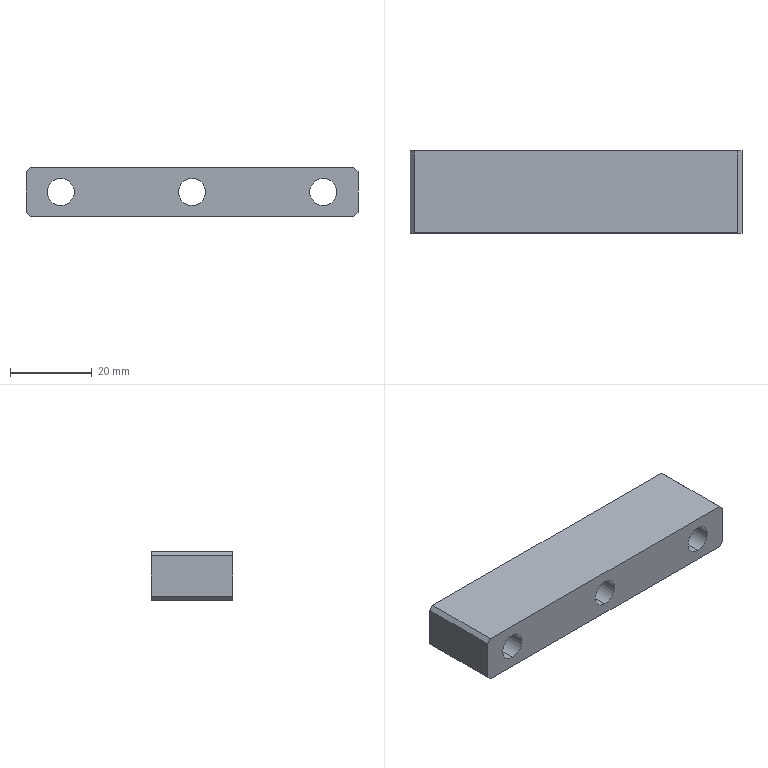Part | SolidWorks | features Chamfer 1, Extrusion 1, HoleWzd 1 | 1 solid | 25 faces | box 81 x 20 x 12 mm | volume 16180 mm3 | plane 13 | cylinder 12 | commonest cylinder face diameters 6.6 x6 11 x6
STEP:
#1=CARTESIAN_POINT('',(-32.,3.6,0.5));
#2=VERTEX_POINT('',#1);
#3=CARTESIAN_POINT('',(-32.,3.6,11.5));
#4=VERTEX_POINT('',#3);
#5=CARTESIAN_POINT('',(-32.,3.6,6.));
#6=DIRECTION('',(0.,1.,0.));
#7=DIRECTION('',(0.,0.,1.));
#8=AXIS2_PLACEMENT_3D('',#5,#6,#7);
#9=CIRCLE('',#8,5.5);
#10=EDGE_CURVE('',#2,#4,#9,.T.);
#11=ORIENTED_EDGE('',*,*,#10,.F.);
#12=CARTESIAN_POINT('',(-32.,10.,0.5));
#13=VERTEX_POINT('',#12);
#14=CARTESIAN_POINT('',(-32.,10.,0.5));
#15=DIRECTION('',(0.,1.,0.));
#16=VECTOR('',#15,1000.);
#17=LINE('',#14,#16);
#18=EDGE_CURVE('',#2,#13,#17,.T.);
#19=ORIENTED_EDGE('',*,*,#18,.T.);
#20=CARTESIAN_POINT('',(-32.,10.,11.5));
#21=VERTEX_POINT('',#20);
#22=CARTESIAN_POINT('',(-32.,10.,6.));
#23=DIRECTION('',(0.,1.,0.));
#24=DIRECTION('',(0.,0.,1.));
#25=AXIS2_PLACEMENT_3D('',#22,#23,#24);
#26=CIRCLE('',#25,5.5);
#27=EDGE_CURVE('',#13,#21,#26,.T.);
#28=ORIENTED_EDGE('',*,*,#27,.T.);
#29=CARTESIAN_POINT('',(-32.,10.,11.5));
#30=DIRECTION('',(0.,1.,0.));
#31=VECTOR('',#30,1000.);
#32=LINE('',#29,#31);
#33=EDGE_CURVE('',#4,#21,#32,.T.);
#34=ORIENTED_EDGE('',*,*,#33,.F.);
#35=EDGE_LOOP('',(#11,#19,#28,#34));
#36=FACE_OUTER_BOUND('',#35,.T.);
#37=CARTESIAN_POINT('',(-32.,10.,6.));
#38=DIRECTION('',(0.,1.,0.));
#39=DIRECTION('',(0.,0.,1.));
#40=AXIS2_PLACEMENT_3D('',#37,#38,#39);
#41=CYLINDRICAL_SURFACE('',#40,5.5);
#42=ADVANCED_FACE('',(#36),#41,.F.);
#43=CARTESIAN_POINT('',(-32.,-10.,2.7));
#44=VERTEX_POINT('',#43);
#45=CARTESIAN_POINT('',(-32.,-10.,9.3));
#46=VERTEX_POINT('',#45);
#47=CARTESIAN_POINT('',(-32.,-10.,6.));
#48=DIRECTION('',(0.,1.,0.));
#49=DIRECTION('',(0.,0.,1.));
#50=AXIS2_PLACEMENT_3D('',#47,#48,#49);
#51=CIRCLE('',#50,3.3);
#52=EDGE_CURVE('',#44,#46,#51,.T.);
#53=ORIENTED_EDGE('',*,*,#52,.F.);
#54=CARTESIAN_POINT('',(-32.,3.6,2.7));
#55=VERTEX_POINT('',#54);
#56=CARTESIAN_POINT('',(-32.,10.,2.7));
#57=DIRECTION('',(0.,1.,0.));
#58=VECTOR('',#57,1000.);
#59=LINE('',#56,#58);
#60=EDGE_CURVE('',#44,#55,#59,.T.);
#61=ORIENTED_EDGE('',*,*,#60,.T.);
#62=CARTESIAN_POINT('',(-32.,3.6,9.3));
#63=VERTEX_POINT('',#62);
#64=CARTESIAN_POINT('',(-32.,3.6,6.));
#65=DIRECTION('',(0.,1.,0.));
#66=DIRECTION('',(0.,0.,1.));
#67=AXIS2_PLACEMENT_3D('',#64,#65,#66);
#68=CIRCLE('',#67,3.3);
#69=EDGE_CURVE('',#55,#63,#68,.T.);
#70=ORIENTED_EDGE('',*,*,#69,.T.);
#71=CARTESIAN_POINT('',(-32.,10.,9.3));
#72=DIRECTION('',(0.,1.,0.));
#73=VECTOR('',#72,1000.);
#74=LINE('',#71,#73);
#75=EDGE_CURVE('',#46,#63,#74,.T.);
#76=ORIENTED_EDGE('',*,*,#75,.F.);
#77=EDGE_LOOP('',(#53,#61,#70,#76));
#78=FACE_OUTER_BOUND('',#77,.T.);
#79=CARTESIAN_POINT('',(-32.,10.,6.));
#80=DIRECTION('',(0.,1.,0.));
#81=DIRECTION('',(0.,0.,1.));
#82=AXIS2_PLACEMENT_3D('',#79,#80,#81);
#83=CYLINDRICAL_SURFACE('',#82,3.3);
#84=ADVANCED_FACE('',(#78),#83,.F.);
#85=CARTESIAN_POINT('',(0.,3.6,0.5));
#86=VERTEX_POINT('',#85);
#87=CARTESIAN_POINT('',(0.,3.6,11.5));
#88=VERTEX_POINT('',#87);
#89=CARTESIAN_POINT('',(0.,3.6,6.));
#90=DIRECTION('',(0.,1.,0.));
#91=DIRECTION('',(0.,0.,1.));
#92=AXIS2_PLACEMENT_3D('',#89,#90,#91);
#93=CIRCLE('',#92,5.5);
#94=EDGE_CURVE('',#86,#88,#93,.T.);
#95=ORIENTED_EDGE('',*,*,#94,.F.);
#96=CARTESIAN_POINT('',(0.,10.,0.5));
#97=VERTEX_POINT('',#96);
#98=CARTESIAN_POINT('',(0.,10.,0.5));
#99=DIRECTION('',(0.,1.,0.));
#100=VECTOR('',#99,1000.);
#101=LINE('',#98,#100);
#102=EDGE_CURVE('',#86,#97,#101,.T.);
#103=ORIENTED_EDGE('',*,*,#102,.T.);
#104=CARTESIAN_POINT('',(0.,10.,11.5));
#105=VERTEX_POINT('',#104);
#106=CARTESIAN_POINT('',(0.,10.,6.));
#107=DIRECTION('',(0.,1.,0.));
#108=DIRECTION('',(0.,0.,1.));
#109=AXIS2_PLACEMENT_3D('',#106,#107,#108);
#110=CIRCLE('',#109,5.5);
#111=EDGE_CURVE('',#97,#105,#110,.T.);
#112=ORIENTED_EDGE('',*,*,#111,.T.);
#113=CARTESIAN_POINT('',(0.,10.,11.5));
#114=DIRECTION('',(0.,1.,0.));
#115=VECTOR('',#114,1000.);
#116=LINE('',#113,#115);
#117=EDGE_CURVE('',#88,#105,#116,.T.);
#118=ORIENTED_EDGE('',*,*,#117,.F.);
#119=EDGE_LOOP('',(#95,#103,#112,#118));
#120=FACE_OUTER_BOUND('',#119,.T.);
#121=CARTESIAN_POINT('',(0.,10.,6.));
#122=DIRECTION('',(0.,1.,0.));
#123=DIRECTION('',(0.,0.,1.));
#124=AXIS2_PLACEMENT_3D('',#121,#122,#123);
#125=CYLINDRICAL_SURFACE('',#124,5.5);
#126=ADVANCED_FACE('',(#120),#125,.F.);
#127=CARTESIAN_POINT('',(0.,-10.,2.7));
#128=VERTEX_POINT('',#127);
#129=CARTESIAN_POINT('',(0.,-10.,9.3));
#130=VERTEX_POINT('',#129);
#131=CARTESIAN_POINT('',(0.,-10.,6.));
#132=DIRECTION('',(0.,1.,0.));
#133=DIRECTION('',(0.,0.,1.));
#134=AXIS2_PLACEMENT_3D('',#131,#132,#133);
#135=CIRCLE('',#134,3.3);
#136=EDGE_CURVE('',#128,#130,#135,.T.);
#137=ORIENTED_EDGE('',*,*,#136,.F.);
#138=CARTESIAN_POINT('',(0.,3.6,2.7));
#139=VERTEX_POINT('',#138);
#140=CARTESIAN_POINT('',(0.,10.,2.7));
#141=DIRECTION('',(0.,1.,0.));
#142=VECTOR('',#141,1000.);
#143=LINE('',#140,#142);
#144=EDGE_CURVE('',#128,#139,#143,.T.);
#145=ORIENTED_EDGE('',*,*,#144,.T.);
#146=CARTESIAN_POINT('',(0.,3.6,9.3));
#147=VERTEX_POINT('',#146);
#148=CARTESIAN_POINT('',(0.,3.6,6.));
#149=DIRECTION('',(0.,1.,0.));
#150=DIRECTION('',(0.,0.,1.));
#151=AXIS2_PLACEMENT_3D('',#148,#149,#150);
#152=CIRCLE('',#151,3.3);
#153=EDGE_CURVE('',#139,#147,#152,.T.);
#154=ORIENTED_EDGE('',*,*,#153,.T.);
#155=CARTESIAN_POINT('',(0.,10.,9.3));
#156=DIRECTION('',(0.,1.,0.));
#157=VECTOR('',#156,1000.);
#158=LINE('',#155,#157);
#159=EDGE_CURVE('',#130,#147,#158,.T.);
#160=ORIENTED_EDGE('',*,*,#159,.F.);
#161=EDGE_LOOP('',(#137,#145,#154,#160));
#162=FACE_OUTER_BOUND('',#161,.T.);
#163=CARTESIAN_POINT('',(0.,10.,6.));
#164=DIRECTION('',(0.,1.,0.));
#165=DIRECTION('',(0.,0.,1.));
#166=AXIS2_PLACEMENT_3D('',#163,#164,#165);
#167=CYLINDRICAL_SURFACE('',#166,3.3);
#168=ADVANCED_FACE('',(#162),#167,.F.);
#169=CARTESIAN_POINT('',(32.,3.6,0.5));
#170=VERTEX_POINT('',#169);
#171=CARTESIAN_POINT('',(32.,3.6,11.5));
#172=VERTEX_POINT('',#171);
#173=CARTESIAN_POINT('',(32.,3.6,6.));
#174=DIRECTION('',(0.,1.,0.));
#175=DIRECTION('',(0.,0.,1.));
#176=AXIS2_PLACEMENT_3D('',#173,#174,#175);
#177=CIRCLE('',#176,5.5);
#178=EDGE_CURVE('',#170,#172,#177,.T.);
#179=ORIENTED_EDGE('',*,*,#178,.F.);
#180=CARTESIAN_POINT('',(32.,10.,0.5));
#181=VERTEX_POINT('',#180);
#182=CARTESIAN_POINT('',(32.,10.,0.5));
#183=DIRECTION('',(0.,1.,0.));
#184=VECTOR('',#183,1000.);
#185=LINE('',#182,#184);
#186=EDGE_CURVE('',#170,#181,#185,.T.);
#187=ORIENTED_EDGE('',*,*,#186,.T.);
#188=CARTESIAN_POINT('',(32.,10.,11.5));
#189=VERTEX_POINT('',#188);
#190=CARTESIAN_POINT('',(32.,10.,6.));
#191=DIRECTION('',(0.,1.,0.));
#192=DIRECTION('',(0.,0.,1.));
#193=AXIS2_PLACEMENT_3D('',#190,#191,#192);
#194=CIRCLE('',#193,5.5);
#195=EDGE_CURVE('',#181,#189,#194,.T.);
#196=ORIENTED_EDGE('',*,*,#195,.T.);
#197=CARTESIAN_POINT('',(32.,10.,11.5));
#198=DIRECTION('',(0.,1.,0.));
#199=VECTOR('',#198,1000.);
#200=LINE('',#197,#199);
#201=EDGE_CURVE('',#172,#189,#200,.T.);
#202=ORIENTED_EDGE('',*,*,#201,.F.);
#203=EDGE_LOOP('',(#179,#187,#196,#202));
#204=FACE_OUTER_BOUND('',#203,.T.);
#205=CARTESIAN_POINT('',(32.,10.,6.));
#206=DIRECTION('',(0.,1.,0.));
#207=DIRECTION('',(0.,0.,1.));
#208=AXIS2_PLACEMENT_3D('',#205,#206,#207);
#209=CYLINDRICAL_SURFACE('',#208,5.5);
#210=ADVANCED_FACE('',(#204),#209,.F.);
#211=CARTESIAN_POINT('',(32.,-10.,2.7));
#212=VERTEX_POINT('',#211);
#213=CARTESIAN_POINT('',(32.,-10.,9.3));
#214=VERTEX_POINT('',#213);
#215=CARTESIAN_POINT('',(32.,-10.,6.));
#216=DIRECTION('',(0.,1.,0.));
#217=DIRECTION('',(0.,0.,1.));
#218=AXIS2_PLACEMENT_3D('',#215,#216,#217);
#219=CIRCLE('',#218,3.3);
#220=EDGE_CURVE('',#212,#214,#219,.T.);
#221=ORIENTED_EDGE('',*,*,#220,.F.);
#222=CARTESIAN_POINT('',(32.,3.6,2.7));
#223=VERTEX_POINT('',#222);
#224=CARTESIAN_POINT('',(32.,10.,2.7));
#225=DIRECTION('',(0.,1.,0.));
#226=VECTOR('',#225,1000.);
#227=LINE('',#224,#226);
#228=EDGE_CURVE('',#212,#223,#227,.T.);
#229=ORIENTED_EDGE('',*,*,#228,.T.);
#230=CARTESIAN_POINT('',(32.,3.6,9.3));
#231=VERTEX_POINT('',#230);
#232=CARTESIAN_POINT('',(32.,3.6,6.));
#233=DIRECTION('',(0.,1.,0.));
#234=DIRECTION('',(0.,0.,1.));
#235=AXIS2_PLACEMENT_3D('',#232,#233,#234);
#236=CIRCLE('',#235,3.3);
#237=EDGE_CURVE('',#223,#231,#236,.T.);
#238=ORIENTED_EDGE('',*,*,#237,.T.);
#239=CARTESIAN_POINT('',(32.,10.,9.3));
#240=DIRECTION('',(0.,1.,0.));
#241=VECTOR('',#240,1000.);
#242=LINE('',#239,#241);
#243=EDGE_CURVE('',#214,#231,#242,.T.);
#244=ORIENTED_EDGE('',*,*,#243,.F.);
#245=EDGE_LOOP('',(#221,#229,#238,#244));
#246=FACE_OUTER_BOUND('',#245,.T.);
#247=CARTESIAN_POINT('',(32.,10.,6.));
#248=DIRECTION('',(0.,1.,0.));
#249=DIRECTION('',(0.,0.,1.));
#250=AXIS2_PLACEMENT_3D('',#247,#248,#249);
#251=CYLINDRICAL_SURFACE('',#250,3.3);
#252=ADVANCED_FACE('',(#246),#251,.F.);
#253=CARTESIAN_POINT('',(40.5,10.,11.));
#254=VERTEX_POINT('',#253);
#255=CARTESIAN_POINT('',(40.5,10.,1.));
#256=VERTEX_POINT('',#255);
#257=CARTESIAN_POINT('',(40.5,10.,12.));
#258=DIRECTION('',(0.,0.,-1.));
#259=VECTOR('',#258,1000.);
#260=LINE('',#257,#259);
#261=EDGE_CURVE('',#254,#256,#260,.T.);
#262=ORIENTED_EDGE('',*,*,#261,.F.);
#263=CARTESIAN_POINT('',(40.5,-10.,11.));
#264=VERTEX_POINT('',#263);
#265=CARTESIAN_POINT('',(40.5,-10.,11.));
#266=DIRECTION('',(0.,-1.,0.));
#267=VECTOR('',#266,1000.);
#268=LINE('',#265,#267);
#269=EDGE_CURVE('',#254,#264,#268,.T.);
#270=ORIENTED_EDGE('',*,*,#269,.T.);
#271=CARTESIAN_POINT('',(40.5,-10.,1.));
#272=VERTEX_POINT('',#271);
#273=CARTESIAN_POINT('',(40.5,-10.,12.));
#274=DIRECTION('',(0.,0.,-1.));
#275=VECTOR('',#274,1000.);
#276=LINE('',#273,#275);
#277=EDGE_CURVE('',#264,#272,#276,.T.);
#278=ORIENTED_EDGE('',*,*,#277,.T.);
#279=CARTESIAN_POINT('',(40.5,10.,1.));
#280=DIRECTION('',(0.,1.,0.));
#281=VECTOR('',#280,1000.);
#282=LINE('',#279,#281);
#283=EDGE_CURVE('',#272,#256,#282,.T.);
#284=ORIENTED_EDGE('',*,*,#283,.T.);
#285=EDGE_LOOP('',(#262,#270,#278,#284));
#286=FACE_OUTER_BOUND('',#285,.T.);
#287=CARTESIAN_POINT('',(40.5,-10.,12.));
#288=DIRECTION('',(-1.,0.,0.));
#289=DIRECTION('',(0.,0.,1.));
#290=AXIS2_PLACEMENT_3D('',#287,#288,#289);
#291=PLANE('',#290);
#292=ADVANCED_FACE('',(#286),#291,.F.);
#293=CARTESIAN_POINT('',(-32.,10.,6.));
#294=DIRECTION('',(0.,1.,0.));
#295=DIRECTION('',(0.,0.,1.));
#296=AXIS2_PLACEMENT_3D('',#293,#294,#295);
#297=CIRCLE('',#296,5.5);
#298=EDGE_CURVE('',#21,#13,#297,.T.);
#299=ORIENTED_EDGE('',*,*,#298,.F.);
#300=ORIENTED_EDGE('',*,*,#27,.F.);
#301=EDGE_LOOP('',(#299,#300));
#302=FACE_BOUND('',#301,.T.);
#303=CARTESIAN_POINT('',(0.,10.,6.));
#304=DIRECTION('',(0.,1.,0.));
#305=DIRECTION('',(0.,0.,1.));
#306=AXIS2_PLACEMENT_3D('',#303,#304,#305);
#307=CIRCLE('',#306,5.5);
#308=EDGE_CURVE('',#105,#97,#307,.T.);
#309=ORIENTED_EDGE('',*,*,#308,.F.);
#310=ORIENTED_EDGE('',*,*,#111,.F.);
#311=EDGE_LOOP('',(#309,#310));
#312=FACE_BOUND('',#311,.T.);
#313=CARTESIAN_POINT('',(32.,10.,6.));
#314=DIRECTION('',(0.,1.,0.));
#315=DIRECTION('',(0.,0.,1.));
#316=AXIS2_PLACEMENT_3D('',#313,#314,#315);
#317=CIRCLE('',#316,5.5);
#318=EDGE_CURVE('',#189,#181,#317,.T.);
#319=ORIENTED_EDGE('',*,*,#318,.F.);
#320=ORIENTED_EDGE('',*,*,#195,.F.);
#321=EDGE_LOOP('',(#319,#320));
#322=FACE_BOUND('',#321,.T.);
#323=CARTESIAN_POINT('',(39.5,10.,12.));
#324=VERTEX_POINT('',#323);
#325=CARTESIAN_POINT('',(-39.5,10.,12.));
#326=VERTEX_POINT('',#325);
#327=CARTESIAN_POINT('',(-40.5,10.,12.));
#328=DIRECTION('',(-1.,0.,0.));
#329=VECTOR('',#328,1000.);
#330=LINE('',#327,#329);
#331=EDGE_CURVE('',#324,#326,#330,.T.);
#332=ORIENTED_EDGE('',*,*,#331,.F.);
#333=CARTESIAN_POINT('',(39.5,10.,12.));
#334=DIRECTION('',(0.7071,0.,-0.7071));
#335=VECTOR('',#334,1000.);
#336=LINE('',#333,#335);
#337=EDGE_CURVE('',#324,#254,#336,.T.);
#338=ORIENTED_EDGE('',*,*,#337,.T.);
#339=ORIENTED_EDGE('',*,*,#261,.T.);
#340=CARTESIAN_POINT('',(39.5,10.,0.));
#341=VERTEX_POINT('',#340);
#342=CARTESIAN_POINT('',(40.5,10.,1.));
#343=DIRECTION('',(-0.7071,0.,-0.7071));
#344=VECTOR('',#343,1000.);
#345=LINE('',#342,#344);
#346=EDGE_CURVE('',#256,#341,#345,.T.);
#347=ORIENTED_EDGE('',*,*,#346,.T.);
#348=CARTESIAN_POINT('',(-39.5,10.,0.));
#349=VERTEX_POINT('',#348);
#350=CARTESIAN_POINT('',(-40.5,10.,0.));
#351=DIRECTION('',(-1.,0.,0.));
#352=VECTOR('',#351,1000.);
#353=LINE('',#350,#352);
#354=EDGE_CURVE('',#341,#349,#353,.T.);
#355=ORIENTED_EDGE('',*,*,#354,.T.);
#356=CARTESIAN_POINT('',(-40.5,10.,1.));
#357=VERTEX_POINT('',#356);
#358=CARTESIAN_POINT('',(-40.5,10.,1.));
#359=DIRECTION('',(-0.7071,0.,0.7071));
#360=VECTOR('',#359,1000.);
#361=LINE('',#358,#360);
#362=EDGE_CURVE('',#349,#357,#361,.T.);
#363=ORIENTED_EDGE('',*,*,#362,.T.);
#364=CARTESIAN_POINT('',(-40.5,10.,11.));
#365=VERTEX_POINT('',#364);
#366=CARTESIAN_POINT('',(-40.5,10.,12.));
#367=DIRECTION('',(0.,0.,-1.));
#368=VECTOR('',#367,1000.);
#369=LINE('',#366,#368);
#370=EDGE_CURVE('',#365,#357,#369,.T.);
#371=ORIENTED_EDGE('',*,*,#370,.F.);
#372=CARTESIAN_POINT('',(-39.5,10.,12.));
#373=DIRECTION('',(0.7071,0.,0.7071));
#374=VECTOR('',#373,1000.);
#375=LINE('',#372,#374);
#376=EDGE_CURVE('',#365,#326,#375,.T.);
#377=ORIENTED_EDGE('',*,*,#376,.T.);
#378=EDGE_LOOP('',(#332,#338,#339,#347,#355,#363,#371,#377));
#379=FACE_OUTER_BOUND('',#378,.T.);
#380=CARTESIAN_POINT('',(-40.5,10.,12.));
#381=DIRECTION('',(0.,-1.,0.));
#382=DIRECTION('',(0.,0.,-1.));
#383=AXIS2_PLACEMENT_3D('',#380,#381,#382);
#384=PLANE('',#383);
#385=ADVANCED_FACE('',(#302,#312,#322,#379),#384,.F.);
#386=ORIENTED_EDGE('',*,*,#370,.T.);
#387=CARTESIAN_POINT('',(-40.5,-10.,1.));
#388=VERTEX_POINT('',#387);
#389=CARTESIAN_POINT('',(-40.5,-10.,1.));
#390=DIRECTION('',(0.,-1.,0.));
#391=VECTOR('',#390,1000.);
#392=LINE('',#389,#391);
#393=EDGE_CURVE('',#357,#388,#392,.T.);
#394=ORIENTED_EDGE('',*,*,#393,.T.);
#395=CARTESIAN_POINT('',(-40.5,-10.,11.));
#396=VERTEX_POINT('',#395);
#397=CARTESIAN_POINT('',(-40.5,-10.,12.));
#398=DIRECTION('',(0.,0.,-1.));
#399=VECTOR('',#398,1000.);
#400=LINE('',#397,#399);
#401=EDGE_CURVE('',#396,#388,#400,.T.);
#402=ORIENTED_EDGE('',*,*,#401,.F.);
#403=CARTESIAN_POINT('',(-40.5,-10.,11.));
#404=DIRECTION('',(0.,1.,0.));
#405=VECTOR('',#404,1000.);
#406=LINE('',#403,#405);
#407=EDGE_CURVE('',#396,#365,#406,.T.);
#408=ORIENTED_EDGE('',*,*,#407,.T.);
#409=EDGE_LOOP('',(#386,#394,#402,#408));
#410=FACE_OUTER_BOUND('',#409,.T.);
#411=CARTESIAN_POINT('',(-40.5,-10.,12.));
#412=DIRECTION('',(1.,0.,0.));
#413=DIRECTION('',(0.,0.,-1.));
#414=AXIS2_PLACEMENT_3D('',#411,#412,#413);
#415=PLANE('',#414);
#416=ADVANCED_FACE('',(#410),#415,.F.);
#417=CARTESIAN_POINT('',(-32.,-10.,6.));
#418=DIRECTION('',(0.,1.,0.));
#419=DIRECTION('',(0.,0.,1.));
#420=AXIS2_PLACEMENT_3D('',#417,#418,#419);
#421=CIRCLE('',#420,3.3);
#422=EDGE_CURVE('',#46,#44,#421,.T.);
#423=ORIENTED_EDGE('',*,*,#422,.T.);
#424=ORIENTED_EDGE('',*,*,#52,.T.);
#425=EDGE_LOOP('',(#423,#424));
#426=FACE_BOUND('',#425,.T.);
#427=CARTESIAN_POINT('',(0.,-10.,6.));
#428=DIRECTION('',(0.,1.,0.));
#429=DIRECTION('',(0.,0.,1.));
#430=AXIS2_PLACEMENT_3D('',#427,#428,#429);
#431=CIRCLE('',#430,3.3);
#432=EDGE_CURVE('',#130,#128,#431,.T.);
#433=ORIENTED_EDGE('',*,*,#432,.T.);
#434=ORIENTED_EDGE('',*,*,#136,.T.);
#435=EDGE_LOOP('',(#433,#434));
#436=FACE_BOUND('',#435,.T.);
#437=CARTESIAN_POINT('',(32.,-10.,6.));
#438=DIRECTION('',(0.,1.,0.));
#439=DIRECTION('',(0.,0.,1.));
#440=AXIS2_PLACEMENT_3D('',#437,#438,#439);
#441=CIRCLE('',#440,3.3);
#442=EDGE_CURVE('',#214,#212,#441,.T.);
#443=ORIENTED_EDGE('',*,*,#442,.T.);
#444=ORIENTED_EDGE('',*,*,#220,.T.);
#445=EDGE_LOOP('',(#443,#444));
#446=FACE_BOUND('',#445,.T.);
#447=ORIENTED_EDGE('',*,*,#277,.F.);
#448=CARTESIAN_POINT('',(39.5,-10.,12.));
#449=VERTEX_POINT('',#448);
#450=CARTESIAN_POINT('',(39.5,-10.,12.));
#451=DIRECTION('',(-0.7071,0.,0.7071));
#452=VECTOR('',#451,1000.);
#453=LINE('',#450,#452);
#454=EDGE_CURVE('',#264,#449,#453,.T.);
#455=ORIENTED_EDGE('',*,*,#454,.T.);
#456=CARTESIAN_POINT('',(-39.5,-10.,12.));
#457=VERTEX_POINT('',#456);
#458=CARTESIAN_POINT('',(-40.5,-10.,12.));
#459=DIRECTION('',(1.,0.,0.));
#460=VECTOR('',#459,1000.);
#461=LINE('',#458,#460);
#462=EDGE_CURVE('',#457,#449,#461,.T.);
#463=ORIENTED_EDGE('',*,*,#462,.F.);
#464=CARTESIAN_POINT('',(-39.5,-10.,12.));
#465=DIRECTION('',(-0.7071,0.,-0.7071));
#466=VECTOR('',#465,1000.);
#467=LINE('',#464,#466);
#468=EDGE_CURVE('',#457,#396,#467,.T.);
#469=ORIENTED_EDGE('',*,*,#468,.T.);
#470=ORIENTED_EDGE('',*,*,#401,.T.);
#471=CARTESIAN_POINT('',(-39.5,-10.,0.));
#472=VERTEX_POINT('',#471);
#473=CARTESIAN_POINT('',(-40.5,-10.,1.));
#474=DIRECTION('',(0.7071,0.,-0.7071));
#475=VECTOR('',#474,1000.);
#476=LINE('',#473,#475);
#477=EDGE_CURVE('',#388,#472,#476,.T.);
#478=ORIENTED_EDGE('',*,*,#477,.T.);
#479=CARTESIAN_POINT('',(39.5,-10.,0.));
#480=VERTEX_POINT('',#479);
#481=CARTESIAN_POINT('',(-40.5,-10.,0.));
#482=DIRECTION('',(1.,0.,0.));
#483=VECTOR('',#482,1000.);
#484=LINE('',#481,#483);
#485=EDGE_CURVE('',#472,#480,#484,.T.);
#486=ORIENTED_EDGE('',*,*,#485,.T.);
#487=CARTESIAN_POINT('',(40.5,-10.,1.));
#488=DIRECTION('',(0.7071,0.,0.7071));
#489=VECTOR('',#488,1000.);
#490=LINE('',#487,#489);
#491=EDGE_CURVE('',#480,#272,#490,.T.);
#492=ORIENTED_EDGE('',*,*,#491,.T.);
#493=EDGE_LOOP('',(#447,#455,#463,#469,#470,#478,#486,#492));
#494=FACE_OUTER_BOUND('',#493,.T.);
#495=CARTESIAN_POINT('',(-40.5,-10.,12.));
#496=DIRECTION('',(0.,1.,0.));
#497=DIRECTION('',(0.,0.,1.));
#498=AXIS2_PLACEMENT_3D('',#495,#496,#497);
#499=PLANE('',#498);
#500=ADVANCED_FACE('',(#426,#436,#446,#494),#499,.F.);
#501=ORIENTED_EDGE('',*,*,#462,.T.);
#502=CARTESIAN_POINT('',(39.5,0.,12.));
#503=DIRECTION('',(0.,1.,0.));
#504=VECTOR('',#503,1000.);
#505=LINE('',#502,#504);
#506=EDGE_CURVE('',#449,#324,#505,.T.);
#507=ORIENTED_EDGE('',*,*,#506,.T.);
#508=ORIENTED_EDGE('',*,*,#331,.T.);
#509=CARTESIAN_POINT('',(-39.5,0.,12.));
#510=DIRECTION('',(0.,-1.,0.));
#511=VECTOR('',#510,1000.);
#512=LINE('',#509,#511);
#513=EDGE_CURVE('',#326,#457,#512,.T.);
#514=ORIENTED_EDGE('',*,*,#513,.T.);
#515=EDGE_LOOP('',(#501,#507,#508,#514));
#516=FACE_OUTER_BOUND('',#515,.T.);
#517=CARTESIAN_POINT('',(0.,0.,12.));
#518=DIRECTION('',(0.,0.,-1.));
#519=DIRECTION('',(-1.,0.,0.));
#520=AXIS2_PLACEMENT_3D('',#517,#518,#519);
#521=PLANE('',#520);
#522=ADVANCED_FACE('',(#516),#521,.F.);
#523=ORIENTED_EDGE('',*,*,#354,.F.);
#524=CARTESIAN_POINT('',(39.5,-10.,0.));
#525=DIRECTION('',(0.,-1.,0.));
#526=VECTOR('',#525,1000.);
#527=LINE('',#524,#526);
#528=EDGE_CURVE('',#341,#480,#527,.T.);
#529=ORIENTED_EDGE('',*,*,#528,.T.);
#530=ORIENTED_EDGE('',*,*,#485,.F.);
#531=CARTESIAN_POINT('',(-39.5,10.,0.));
#532=DIRECTION('',(0.,1.,0.));
#533=VECTOR('',#532,1000.);
#534=LINE('',#531,#533);
#535=EDGE_CURVE('',#472,#349,#534,.T.);
#536=ORIENTED_EDGE('',*,*,#535,.T.);
#537=EDGE_LOOP('',(#523,#529,#530,#536));
#538=FACE_OUTER_BOUND('',#537,.T.);
#539=CARTESIAN_POINT('',(0.,0.,0.));
#540=DIRECTION('',(0.,0.,-1.));
#541=DIRECTION('',(-1.,0.,0.));
#542=AXIS2_PLACEMENT_3D('',#539,#540,#541);
#543=PLANE('',#542);
#544=ADVANCED_FACE('',(#538),#543,.T.);
#545=ORIENTED_EDGE('',*,*,#228,.F.);
#546=ORIENTED_EDGE('',*,*,#442,.F.);
#547=ORIENTED_EDGE('',*,*,#243,.T.);
#548=CARTESIAN_POINT('',(32.,3.6,6.));
#549=DIRECTION('',(0.,1.,0.));
#550=DIRECTION('',(0.,0.,1.));
#551=AXIS2_PLACEMENT_3D('',#548,#549,#550);
#552=CIRCLE('',#551,3.3);
#553=EDGE_CURVE('',#231,#223,#552,.T.);
#554=ORIENTED_EDGE('',*,*,#553,.T.);
#555=EDGE_LOOP('',(#545,#546,#547,#554));
#556=FACE_OUTER_BOUND('',#555,.T.);
#557=CARTESIAN_POINT('',(32.,10.,6.));
#558=DIRECTION('',(0.,1.,0.));
#559=DIRECTION('',(0.,0.,1.));
#560=AXIS2_PLACEMENT_3D('',#557,#558,#559);
#561=CYLINDRICAL_SURFACE('',#560,3.3);
#562=ADVANCED_FACE('',(#556),#561,.F.);
#563=ORIENTED_EDGE('',*,*,#553,.F.);
#564=ORIENTED_EDGE('',*,*,#237,.F.);
#565=EDGE_LOOP('',(#563,#564));
#566=FACE_BOUND('',#565,.T.);
#567=CARTESIAN_POINT('',(32.,3.6,6.));
#568=DIRECTION('',(0.,1.,0.));
#569=DIRECTION('',(0.,0.,1.));
#570=AXIS2_PLACEMENT_3D('',#567,#568,#569);
#571=CIRCLE('',#570,5.5);
#572=EDGE_CURVE('',#172,#170,#571,.T.);
#573=ORIENTED_EDGE('',*,*,#572,.T.);
#574=ORIENTED_EDGE('',*,*,#178,.T.);
#575=EDGE_LOOP('',(#573,#574));
#576=FACE_OUTER_BOUND('',#575,.T.);
#577=CARTESIAN_POINT('',(35.3,3.6,6.));
#578=DIRECTION('',(0.,-1.,0.));
#579=DIRECTION('',(0.,0.,-1.));
#580=AXIS2_PLACEMENT_3D('',#577,#578,#579);
#581=PLANE('',#580);
#582=ADVANCED_FACE('',(#566,#576),#581,.F.);
#583=ORIENTED_EDGE('',*,*,#186,.F.);
#584=ORIENTED_EDGE('',*,*,#572,.F.);
#585=ORIENTED_EDGE('',*,*,#201,.T.);
#586=ORIENTED_EDGE('',*,*,#318,.T.);
#587=EDGE_LOOP('',(#583,#584,#585,#586));
#588=FACE_OUTER_BOUND('',#587,.T.);
#589=CARTESIAN_POINT('',(32.,10.,6.));
#590=DIRECTION('',(0.,1.,0.));
#591=DIRECTION('',(0.,0.,1.));
#592=AXIS2_PLACEMENT_3D('',#589,#590,#591);
#593=CYLINDRICAL_SURFACE('',#592,5.5);
#594=ADVANCED_FACE('',(#588),#593,.F.);
#595=ORIENTED_EDGE('',*,*,#144,.F.);
#596=ORIENTED_EDGE('',*,*,#432,.F.);
#597=ORIENTED_EDGE('',*,*,#159,.T.);
#598=CARTESIAN_POINT('',(0.,3.6,6.));
#599=DIRECTION('',(0.,1.,0.));
#600=DIRECTION('',(0.,0.,1.));
#601=AXIS2_PLACEMENT_3D('',#598,#599,#600);
#602=CIRCLE('',#601,3.3);
#603=EDGE_CURVE('',#147,#139,#602,.T.);
#604=ORIENTED_EDGE('',*,*,#603,.T.);
#605=EDGE_LOOP('',(#595,#596,#597,#604));
#606=FACE_OUTER_BOUND('',#605,.T.);
#607=CARTESIAN_POINT('',(0.,10.,6.));
#608=DIRECTION('',(0.,1.,0.));
#609=DIRECTION('',(0.,0.,1.));
#610=AXIS2_PLACEMENT_3D('',#607,#608,#609);
#611=CYLINDRICAL_SURFACE('',#610,3.3);
#612=ADVANCED_FACE('',(#606),#611,.F.);
#613=ORIENTED_EDGE('',*,*,#603,.F.);
#614=ORIENTED_EDGE('',*,*,#153,.F.);
#615=EDGE_LOOP('',(#613,#614));
#616=FACE_BOUND('',#615,.T.);
#617=CARTESIAN_POINT('',(0.,3.6,6.));
#618=DIRECTION('',(0.,1.,0.));
#619=DIRECTION('',(0.,0.,1.));
#620=AXIS2_PLACEMENT_3D('',#617,#618,#619);
#621=CIRCLE('',#620,5.5);
#622=EDGE_CURVE('',#88,#86,#621,.T.);
#623=ORIENTED_EDGE('',*,*,#622,.T.);
#624=ORIENTED_EDGE('',*,*,#94,.T.);
#625=EDGE_LOOP('',(#623,#624));
#626=FACE_OUTER_BOUND('',#625,.T.);
#627=CARTESIAN_POINT('',(3.3,3.6,6.));
#628=DIRECTION('',(0.,-1.,0.));
#629=DIRECTION('',(0.,0.,-1.));
#630=AXIS2_PLACEMENT_3D('',#627,#628,#629);
#631=PLANE('',#630);
#632=ADVANCED_FACE('',(#616,#626),#631,.F.);
#633=ORIENTED_EDGE('',*,*,#102,.F.);
#634=ORIENTED_EDGE('',*,*,#622,.F.);
#635=ORIENTED_EDGE('',*,*,#117,.T.);
#636=ORIENTED_EDGE('',*,*,#308,.T.);
#637=EDGE_LOOP('',(#633,#634,#635,#636));
#638=FACE_OUTER_BOUND('',#637,.T.);
#639=CARTESIAN_POINT('',(0.,10.,6.));
#640=DIRECTION('',(0.,1.,0.));
#641=DIRECTION('',(0.,0.,1.));
#642=AXIS2_PLACEMENT_3D('',#639,#640,#641);
#643=CYLINDRICAL_SURFACE('',#642,5.5);
#644=ADVANCED_FACE('',(#638),#643,.F.);
#645=ORIENTED_EDGE('',*,*,#60,.F.);
#646=ORIENTED_EDGE('',*,*,#422,.F.);
#647=ORIENTED_EDGE('',*,*,#75,.T.);
#648=CARTESIAN_POINT('',(-32.,3.6,6.));
#649=DIRECTION('',(0.,1.,0.));
#650=DIRECTION('',(0.,0.,1.));
#651=AXIS2_PLACEMENT_3D('',#648,#649,#650);
#652=CIRCLE('',#651,3.3);
#653=EDGE_CURVE('',#63,#55,#652,.T.);
#654=ORIENTED_EDGE('',*,*,#653,.T.);
#655=EDGE_LOOP('',(#645,#646,#647,#654));
#656=FACE_OUTER_BOUND('',#655,.T.);
#657=CARTESIAN_POINT('',(-32.,10.,6.));
#658=DIRECTION('',(0.,1.,0.));
#659=DIRECTION('',(0.,0.,1.));
#660=AXIS2_PLACEMENT_3D('',#657,#658,#659);
#661=CYLINDRICAL_SURFACE('',#660,3.3);
#662=ADVANCED_FACE('',(#656),#661,.F.);
#663=ORIENTED_EDGE('',*,*,#653,.F.);
#664=ORIENTED_EDGE('',*,*,#69,.F.);
#665=EDGE_LOOP('',(#663,#664));
#666=FACE_BOUND('',#665,.T.);
#667=CARTESIAN_POINT('',(-32.,3.6,6.));
#668=DIRECTION('',(0.,1.,0.));
#669=DIRECTION('',(0.,0.,1.));
#670=AXIS2_PLACEMENT_3D('',#667,#668,#669);
#671=CIRCLE('',#670,5.5);
#672=EDGE_CURVE('',#4,#2,#671,.T.);
#673=ORIENTED_EDGE('',*,*,#672,.T.);
#674=ORIENTED_EDGE('',*,*,#10,.T.);
#675=EDGE_LOOP('',(#673,#674));
#676=FACE_OUTER_BOUND('',#675,.T.);
#677=CARTESIAN_POINT('',(-28.7,3.6,6.));
#678=DIRECTION('',(0.,-1.,0.));
#679=DIRECTION('',(0.,0.,-1.));
#680=AXIS2_PLACEMENT_3D('',#677,#678,#679);
#681=PLANE('',#680);
#682=ADVANCED_FACE('',(#666,#676),#681,.F.);
#683=ORIENTED_EDGE('',*,*,#18,.F.);
#684=ORIENTED_EDGE('',*,*,#672,.F.);
#685=ORIENTED_EDGE('',*,*,#33,.T.);
#686=ORIENTED_EDGE('',*,*,#298,.T.);
#687=EDGE_LOOP('',(#683,#684,#685,#686));
#688=FACE_OUTER_BOUND('',#687,.T.);
#689=CARTESIAN_POINT('',(-32.,10.,6.));
#690=DIRECTION('',(0.,1.,0.));
#691=DIRECTION('',(0.,0.,1.));
#692=AXIS2_PLACEMENT_3D('',#689,#690,#691);
#693=CYLINDRICAL_SURFACE('',#692,5.5);
#694=ADVANCED_FACE('',(#688),#693,.F.);
#695=ORIENTED_EDGE('',*,*,#454,.F.);
#696=ORIENTED_EDGE('',*,*,#269,.F.);
#697=ORIENTED_EDGE('',*,*,#337,.F.);
#698=ORIENTED_EDGE('',*,*,#506,.F.);
#699=EDGE_LOOP('',(#695,#696,#697,#698));
#700=FACE_OUTER_BOUND('',#699,.T.);
#701=CARTESIAN_POINT('',(39.5,0.,12.));
#702=DIRECTION('',(-0.7071,0.,-0.7071));
#703=DIRECTION('',(0.,1.,0.));
#704=AXIS2_PLACEMENT_3D('',#701,#702,#703);
#705=PLANE('',#704);
#706=ADVANCED_FACE('',(#700),#705,.F.);
#707=ORIENTED_EDGE('',*,*,#491,.F.);
#708=ORIENTED_EDGE('',*,*,#528,.F.);
#709=ORIENTED_EDGE('',*,*,#346,.F.);
#710=ORIENTED_EDGE('',*,*,#283,.F.);
#711=EDGE_LOOP('',(#707,#708,#709,#710));
#712=FACE_OUTER_BOUND('',#711,.T.);
#713=CARTESIAN_POINT('',(40.5,-10.,1.));
#714=DIRECTION('',(0.7071,0.,-0.7071));
#715=DIRECTION('',(0.,-1.,0.));
#716=AXIS2_PLACEMENT_3D('',#713,#714,#715);
#717=PLANE('',#716);
#718=ADVANCED_FACE('',(#712),#717,.T.);
#719=ORIENTED_EDGE('',*,*,#362,.F.);
#720=ORIENTED_EDGE('',*,*,#535,.F.);
#721=ORIENTED_EDGE('',*,*,#477,.F.);
#722=ORIENTED_EDGE('',*,*,#393,.F.);
#723=EDGE_LOOP('',(#719,#720,#721,#722));
#724=FACE_OUTER_BOUND('',#723,.T.);
#725=CARTESIAN_POINT('',(-40.5,-10.,1.));
#726=DIRECTION('',(-0.7071,0.,-0.7071));
#727=DIRECTION('',(0.,1.,0.));
#728=AXIS2_PLACEMENT_3D('',#725,#726,#727);
#729=PLANE('',#728);
#730=ADVANCED_FACE('',(#724),#729,.T.);
#731=ORIENTED_EDGE('',*,*,#376,.F.);
#732=ORIENTED_EDGE('',*,*,#407,.F.);
#733=ORIENTED_EDGE('',*,*,#468,.F.);
#734=ORIENTED_EDGE('',*,*,#513,.F.);
#735=EDGE_LOOP('',(#731,#732,#733,#734));
#736=FACE_OUTER_BOUND('',#735,.T.);
#737=CARTESIAN_POINT('',(-39.5,0.,12.));
#738=DIRECTION('',(0.7071,0.,-0.7071));
#739=DIRECTION('',(0.,-1.,0.));
#740=AXIS2_PLACEMENT_3D('',#737,#738,#739);
#741=PLANE('',#740);
#742=ADVANCED_FACE('',(#736),#741,.F.);
#743=CLOSED_SHELL('',(#42,#84,#126,#168,#210,#252,#292,#385,#416,#500,#522,#544,#562,#582,#594,#612,#632,#644,#662,#682,#694,#706,#718,#730,#742));
#744=MANIFOLD_SOLID_BREP('',#743);
#745=CARTESIAN_POINT('',(0.,0.,0.));
#746=DIRECTION('',(0.,0.,1.));
#747=DIRECTION('',(1.,0.,0.));
#748=AXIS2_PLACEMENT_3D('',#745,#746,#747);
#749=(LENGTH_UNIT()NAMED_UNIT(*)SI_UNIT(.MILLI.,.METRE.));
#750=UNCERTAINTY_MEASURE_WITH_UNIT(LENGTH_MEASURE(0.00001),#749,'','');
#751=(NAMED_UNIT(*)PLANE_ANGLE_UNIT()SI_UNIT($,.RADIAN.));
#752=(NAMED_UNIT(*)SI_UNIT($,.STERADIAN.)SOLID_ANGLE_UNIT());
#753=(GEOMETRIC_REPRESENTATION_CONTEXT(3)GLOBAL_UNCERTAINTY_ASSIGNED_CONTEXT((#750))GLOBAL_UNIT_ASSIGNED_CONTEXT((#749,#751,#752))REPRESENTATION_CONTEXT('',''));
#754=ADVANCED_BREP_SHAPE_REPRESENTATION('',(#744,#748),#753);